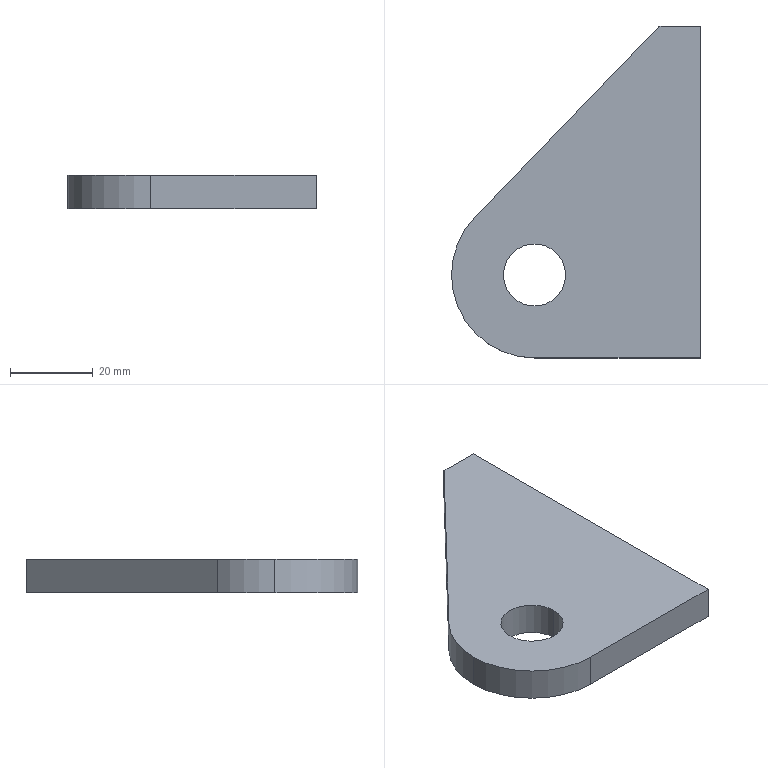Part | SolidWorks | features Extrusion 1 | 1 solid | 10 faces | box 60 x 80 x 8 mm | volume 25848 mm3 | plane 6 | cylinder 4 | commonest cylinder face diameters 15 x2 40 x2
STEP:
#1=CARTESIAN_POINT('',(-47.5,20.,4.));
#2=VERTEX_POINT('',#1);
#3=CARTESIAN_POINT('',(-32.5,20.,4.));
#4=VERTEX_POINT('',#3);
#5=CARTESIAN_POINT('',(-40.,20.,4.));
#6=DIRECTION('',(0.,0.,1.));
#7=DIRECTION('',(1.,0.,0.));
#8=AXIS2_PLACEMENT_3D('',#5,#6,#7);
#9=CIRCLE('',#8,7.5);
#10=EDGE_CURVE('',#2,#4,#9,.T.);
#11=ORIENTED_EDGE('',*,*,#10,.T.);
#12=CARTESIAN_POINT('',(-32.5,20.,-4.));
#13=VERTEX_POINT('',#12);
#14=CARTESIAN_POINT('',(-32.5,20.,4.));
#15=DIRECTION('',(0.,0.,-1.));
#16=VECTOR('',#15,1000.);
#17=LINE('',#14,#16);
#18=EDGE_CURVE('',#4,#13,#17,.T.);
#19=ORIENTED_EDGE('',*,*,#18,.T.);
#20=CARTESIAN_POINT('',(-47.5,20.,-4.));
#21=VERTEX_POINT('',#20);
#22=CARTESIAN_POINT('',(-40.,20.,-4.));
#23=DIRECTION('',(0.,0.,1.));
#24=DIRECTION('',(1.,0.,0.));
#25=AXIS2_PLACEMENT_3D('',#22,#23,#24);
#26=CIRCLE('',#25,7.5);
#27=EDGE_CURVE('',#21,#13,#26,.T.);
#28=ORIENTED_EDGE('',*,*,#27,.F.);
#29=CARTESIAN_POINT('',(-47.5,20.,4.));
#30=DIRECTION('',(0.,0.,-1.));
#31=VECTOR('',#30,1000.);
#32=LINE('',#29,#31);
#33=EDGE_CURVE('',#2,#21,#32,.T.);
#34=ORIENTED_EDGE('',*,*,#33,.F.);
#35=EDGE_LOOP('',(#11,#19,#28,#34));
#36=FACE_OUTER_BOUND('',#35,.T.);
#37=CARTESIAN_POINT('',(-40.,20.,4.));
#38=DIRECTION('',(0.,0.,-1.));
#39=DIRECTION('',(-1.,0.,0.));
#40=AXIS2_PLACEMENT_3D('',#37,#38,#39);
#41=CYLINDRICAL_SURFACE('',#40,7.5);
#42=ADVANCED_FACE('',(#36),#41,.F.);
#43=CARTESIAN_POINT('',(-60.,20.,4.));
#44=VERTEX_POINT('',#43);
#45=CARTESIAN_POINT('',(-40.,0.,4.));
#46=VERTEX_POINT('',#45);
#47=CARTESIAN_POINT('',(-40.,20.,4.));
#48=DIRECTION('',(0.,0.,1.));
#49=DIRECTION('',(1.,0.,0.));
#50=AXIS2_PLACEMENT_3D('',#47,#48,#49);
#51=CIRCLE('',#50,20.);
#52=EDGE_CURVE('',#44,#46,#51,.T.);
#53=ORIENTED_EDGE('',*,*,#52,.F.);
#54=CARTESIAN_POINT('',(-60.,20.,-4.));
#55=VERTEX_POINT('',#54);
#56=CARTESIAN_POINT('',(-60.,20.,4.));
#57=DIRECTION('',(0.,0.,-1.));
#58=VECTOR('',#57,1000.);
#59=LINE('',#56,#58);
#60=EDGE_CURVE('',#44,#55,#59,.T.);
#61=ORIENTED_EDGE('',*,*,#60,.T.);
#62=CARTESIAN_POINT('',(-40.,0.,-4.));
#63=VERTEX_POINT('',#62);
#64=CARTESIAN_POINT('',(-40.,20.,-4.));
#65=DIRECTION('',(0.,0.,1.));
#66=DIRECTION('',(1.,0.,0.));
#67=AXIS2_PLACEMENT_3D('',#64,#65,#66);
#68=CIRCLE('',#67,20.);
#69=EDGE_CURVE('',#55,#63,#68,.T.);
#70=ORIENTED_EDGE('',*,*,#69,.T.);
#71=CARTESIAN_POINT('',(-40.,0.,4.));
#72=DIRECTION('',(0.,0.,-1.));
#73=VECTOR('',#72,1000.);
#74=LINE('',#71,#73);
#75=EDGE_CURVE('',#46,#63,#74,.T.);
#76=ORIENTED_EDGE('',*,*,#75,.F.);
#77=EDGE_LOOP('',(#53,#61,#70,#76));
#78=FACE_OUTER_BOUND('',#77,.T.);
#79=CARTESIAN_POINT('',(-40.,20.,4.));
#80=DIRECTION('',(0.,0.,-1.));
#81=DIRECTION('',(-1.,0.,0.));
#82=AXIS2_PLACEMENT_3D('',#79,#80,#81);
#83=CYLINDRICAL_SURFACE('',#82,20.);
#84=ADVANCED_FACE('',(#78),#83,.T.);
#85=CARTESIAN_POINT('',(0.,0.,4.));
#86=VERTEX_POINT('',#85);
#87=CARTESIAN_POINT('',(-40.,0.,4.));
#88=DIRECTION('',(1.,0.,0.));
#89=VECTOR('',#88,1000.);
#90=LINE('',#87,#89);
#91=EDGE_CURVE('',#46,#86,#90,.T.);
#92=ORIENTED_EDGE('',*,*,#91,.T.);
#93=CARTESIAN_POINT('',(0.,80.,4.));
#94=VERTEX_POINT('',#93);
#95=CARTESIAN_POINT('',(0.,0.,4.));
#96=DIRECTION('',(0.,1.,0.));
#97=VECTOR('',#96,1000.);
#98=LINE('',#95,#97);
#99=EDGE_CURVE('',#86,#94,#98,.T.);
#100=ORIENTED_EDGE('',*,*,#99,.T.);
#101=CARTESIAN_POINT('',(-10.,80.,4.));
#102=VERTEX_POINT('',#101);
#103=CARTESIAN_POINT('',(0.,80.,4.));
#104=DIRECTION('',(-1.,0.,0.));
#105=VECTOR('',#104,1000.);
#106=LINE('',#103,#105);
#107=EDGE_CURVE('',#94,#102,#106,.T.);
#108=ORIENTED_EDGE('',*,*,#107,.T.);
#109=CARTESIAN_POINT('',(-54.408,33.871,4.));
#110=VERTEX_POINT('',#109);
#111=CARTESIAN_POINT('',(-10.,80.,4.));
#112=DIRECTION('',(-0.6935,-0.7204,0.));
#113=VECTOR('',#112,1000.);
#114=LINE('',#111,#113);
#115=EDGE_CURVE('',#102,#110,#114,.T.);
#116=ORIENTED_EDGE('',*,*,#115,.T.);
#117=CARTESIAN_POINT('',(-40.,20.,4.));
#118=DIRECTION('',(0.,0.,1.));
#119=DIRECTION('',(1.,0.,0.));
#120=AXIS2_PLACEMENT_3D('',#117,#118,#119);
#121=CIRCLE('',#120,20.);
#122=EDGE_CURVE('',#110,#44,#121,.T.);
#123=ORIENTED_EDGE('',*,*,#122,.T.);
#124=ORIENTED_EDGE('',*,*,#52,.T.);
#125=EDGE_LOOP('',(#92,#100,#108,#116,#123,#124));
#126=FACE_OUTER_BOUND('',#125,.T.);
#127=ORIENTED_EDGE('',*,*,#10,.F.);
#128=CARTESIAN_POINT('',(-40.,20.,4.));
#129=DIRECTION('',(0.,0.,1.));
#130=DIRECTION('',(1.,0.,0.));
#131=AXIS2_PLACEMENT_3D('',#128,#129,#130);
#132=CIRCLE('',#131,7.5);
#133=EDGE_CURVE('',#4,#2,#132,.T.);
#134=ORIENTED_EDGE('',*,*,#133,.F.);
#135=EDGE_LOOP('',(#127,#134));
#136=FACE_BOUND('',#135,.T.);
#137=CARTESIAN_POINT('',(-40.,20.,4.));
#138=DIRECTION('',(0.,0.,1.));
#139=DIRECTION('',(1.,0.,0.));
#140=AXIS2_PLACEMENT_3D('',#137,#138,#139);
#141=PLANE('',#140);
#142=ADVANCED_FACE('',(#126,#136),#141,.T.);
#143=CARTESIAN_POINT('',(0.,0.,-4.));
#144=VERTEX_POINT('',#143);
#145=CARTESIAN_POINT('',(-40.,0.,-4.));
#146=DIRECTION('',(1.,0.,0.));
#147=VECTOR('',#146,1000.);
#148=LINE('',#145,#147);
#149=EDGE_CURVE('',#63,#144,#148,.T.);
#150=ORIENTED_EDGE('',*,*,#149,.F.);
#151=ORIENTED_EDGE('',*,*,#69,.F.);
#152=CARTESIAN_POINT('',(-54.408,33.871,-4.));
#153=VERTEX_POINT('',#152);
#154=CARTESIAN_POINT('',(-40.,20.,-4.));
#155=DIRECTION('',(0.,0.,1.));
#156=DIRECTION('',(1.,0.,0.));
#157=AXIS2_PLACEMENT_3D('',#154,#155,#156);
#158=CIRCLE('',#157,20.);
#159=EDGE_CURVE('',#153,#55,#158,.T.);
#160=ORIENTED_EDGE('',*,*,#159,.F.);
#161=CARTESIAN_POINT('',(-10.,80.,-4.));
#162=VERTEX_POINT('',#161);
#163=CARTESIAN_POINT('',(-10.,80.,-4.));
#164=DIRECTION('',(-0.6935,-0.7204,0.));
#165=VECTOR('',#164,1000.);
#166=LINE('',#163,#165);
#167=EDGE_CURVE('',#162,#153,#166,.T.);
#168=ORIENTED_EDGE('',*,*,#167,.F.);
#169=CARTESIAN_POINT('',(0.,80.,-4.));
#170=VERTEX_POINT('',#169);
#171=CARTESIAN_POINT('',(0.,80.,-4.));
#172=DIRECTION('',(-1.,0.,0.));
#173=VECTOR('',#172,1000.);
#174=LINE('',#171,#173);
#175=EDGE_CURVE('',#170,#162,#174,.T.);
#176=ORIENTED_EDGE('',*,*,#175,.F.);
#177=CARTESIAN_POINT('',(0.,0.,-4.));
#178=DIRECTION('',(0.,1.,0.));
#179=VECTOR('',#178,1000.);
#180=LINE('',#177,#179);
#181=EDGE_CURVE('',#144,#170,#180,.T.);
#182=ORIENTED_EDGE('',*,*,#181,.F.);
#183=EDGE_LOOP('',(#150,#151,#160,#168,#176,#182));
#184=FACE_OUTER_BOUND('',#183,.T.);
#185=ORIENTED_EDGE('',*,*,#27,.T.);
#186=CARTESIAN_POINT('',(-40.,20.,-4.));
#187=DIRECTION('',(0.,0.,1.));
#188=DIRECTION('',(1.,0.,0.));
#189=AXIS2_PLACEMENT_3D('',#186,#187,#188);
#190=CIRCLE('',#189,7.5);
#191=EDGE_CURVE('',#13,#21,#190,.T.);
#192=ORIENTED_EDGE('',*,*,#191,.T.);
#193=EDGE_LOOP('',(#185,#192));
#194=FACE_BOUND('',#193,.T.);
#195=CARTESIAN_POINT('',(-40.,20.,-4.));
#196=DIRECTION('',(0.,0.,1.));
#197=DIRECTION('',(1.,0.,0.));
#198=AXIS2_PLACEMENT_3D('',#195,#196,#197);
#199=PLANE('',#198);
#200=ADVANCED_FACE('',(#184,#194),#199,.F.);
#201=ORIENTED_EDGE('',*,*,#149,.T.);
#202=CARTESIAN_POINT('',(0.,0.,4.));
#203=DIRECTION('',(0.,0.,-1.));
#204=VECTOR('',#203,1000.);
#205=LINE('',#202,#204);
#206=EDGE_CURVE('',#86,#144,#205,.T.);
#207=ORIENTED_EDGE('',*,*,#206,.F.);
#208=ORIENTED_EDGE('',*,*,#91,.F.);
#209=ORIENTED_EDGE('',*,*,#75,.T.);
#210=EDGE_LOOP('',(#201,#207,#208,#209));
#211=FACE_OUTER_BOUND('',#210,.T.);
#212=CARTESIAN_POINT('',(-40.,0.,4.));
#213=DIRECTION('',(0.,1.,0.));
#214=DIRECTION('',(0.,0.,1.));
#215=AXIS2_PLACEMENT_3D('',#212,#213,#214);
#216=PLANE('',#215);
#217=ADVANCED_FACE('',(#211),#216,.F.);
#218=ORIENTED_EDGE('',*,*,#181,.T.);
#219=CARTESIAN_POINT('',(0.,80.,4.));
#220=DIRECTION('',(0.,0.,-1.));
#221=VECTOR('',#220,1000.);
#222=LINE('',#219,#221);
#223=EDGE_CURVE('',#94,#170,#222,.T.);
#224=ORIENTED_EDGE('',*,*,#223,.F.);
#225=ORIENTED_EDGE('',*,*,#99,.F.);
#226=ORIENTED_EDGE('',*,*,#206,.T.);
#227=EDGE_LOOP('',(#218,#224,#225,#226));
#228=FACE_OUTER_BOUND('',#227,.T.);
#229=CARTESIAN_POINT('',(0.,0.,4.));
#230=DIRECTION('',(-1.,0.,0.));
#231=DIRECTION('',(0.,0.,1.));
#232=AXIS2_PLACEMENT_3D('',#229,#230,#231);
#233=PLANE('',#232);
#234=ADVANCED_FACE('',(#228),#233,.F.);
#235=ORIENTED_EDGE('',*,*,#175,.T.);
#236=CARTESIAN_POINT('',(-10.,80.,4.));
#237=DIRECTION('',(0.,0.,-1.));
#238=VECTOR('',#237,1000.);
#239=LINE('',#236,#238);
#240=EDGE_CURVE('',#102,#162,#239,.T.);
#241=ORIENTED_EDGE('',*,*,#240,.F.);
#242=ORIENTED_EDGE('',*,*,#107,.F.);
#243=ORIENTED_EDGE('',*,*,#223,.T.);
#244=EDGE_LOOP('',(#235,#241,#242,#243));
#245=FACE_OUTER_BOUND('',#244,.T.);
#246=CARTESIAN_POINT('',(0.,80.,4.));
#247=DIRECTION('',(0.,-1.,0.));
#248=DIRECTION('',(0.,0.,-1.));
#249=AXIS2_PLACEMENT_3D('',#246,#247,#248);
#250=PLANE('',#249);
#251=ADVANCED_FACE('',(#245),#250,.F.);
#252=ORIENTED_EDGE('',*,*,#167,.T.);
#253=CARTESIAN_POINT('',(-54.408,33.871,4.));
#254=DIRECTION('',(0.,0.,-1.));
#255=VECTOR('',#254,1000.);
#256=LINE('',#253,#255);
#257=EDGE_CURVE('',#110,#153,#256,.T.);
#258=ORIENTED_EDGE('',*,*,#257,.F.);
#259=ORIENTED_EDGE('',*,*,#115,.F.);
#260=ORIENTED_EDGE('',*,*,#240,.T.);
#261=EDGE_LOOP('',(#252,#258,#259,#260));
#262=FACE_OUTER_BOUND('',#261,.T.);
#263=CARTESIAN_POINT('',(-10.,80.,4.));
#264=DIRECTION('',(0.7204,-0.6935,0.));
#265=DIRECTION('',(0.6935,0.7204,0.));
#266=AXIS2_PLACEMENT_3D('',#263,#264,#265);
#267=PLANE('',#266);
#268=ADVANCED_FACE('',(#262),#267,.F.);
#269=ORIENTED_EDGE('',*,*,#60,.F.);
#270=ORIENTED_EDGE('',*,*,#122,.F.);
#271=ORIENTED_EDGE('',*,*,#257,.T.);
#272=ORIENTED_EDGE('',*,*,#159,.T.);
#273=EDGE_LOOP('',(#269,#270,#271,#272));
#274=FACE_OUTER_BOUND('',#273,.T.);
#275=CARTESIAN_POINT('',(-40.,20.,4.));
#276=DIRECTION('',(0.,0.,-1.));
#277=DIRECTION('',(-1.,0.,0.));
#278=AXIS2_PLACEMENT_3D('',#275,#276,#277);
#279=CYLINDRICAL_SURFACE('',#278,20.);
#280=ADVANCED_FACE('',(#274),#279,.T.);
#281=ORIENTED_EDGE('',*,*,#18,.F.);
#282=ORIENTED_EDGE('',*,*,#133,.T.);
#283=ORIENTED_EDGE('',*,*,#33,.T.);
#284=ORIENTED_EDGE('',*,*,#191,.F.);
#285=EDGE_LOOP('',(#281,#282,#283,#284));
#286=FACE_OUTER_BOUND('',#285,.T.);
#287=CARTESIAN_POINT('',(-40.,20.,4.));
#288=DIRECTION('',(0.,0.,-1.));
#289=DIRECTION('',(-1.,0.,0.));
#290=AXIS2_PLACEMENT_3D('',#287,#288,#289);
#291=CYLINDRICAL_SURFACE('',#290,7.5);
#292=ADVANCED_FACE('',(#286),#291,.F.);
#293=CLOSED_SHELL('',(#42,#84,#142,#200,#217,#234,#251,#268,#280,#292));
#294=MANIFOLD_SOLID_BREP('',#293);
#295=CARTESIAN_POINT('',(0.,0.,0.));
#296=DIRECTION('',(0.,0.,1.));
#297=DIRECTION('',(1.,0.,0.));
#298=AXIS2_PLACEMENT_3D('',#295,#296,#297);
#299=(LENGTH_UNIT()NAMED_UNIT(*)SI_UNIT(.MILLI.,.METRE.));
#300=UNCERTAINTY_MEASURE_WITH_UNIT(LENGTH_MEASURE(0.00001),#299,'','');
#301=(NAMED_UNIT(*)PLANE_ANGLE_UNIT()SI_UNIT($,.RADIAN.));
#302=(NAMED_UNIT(*)SI_UNIT($,.STERADIAN.)SOLID_ANGLE_UNIT());
#303=(GEOMETRIC_REPRESENTATION_CONTEXT(3)GLOBAL_UNCERTAINTY_ASSIGNED_CONTEXT((#300))GLOBAL_UNIT_ASSIGNED_CONTEXT((#299,#301,#302))REPRESENTATION_CONTEXT('',''));
#304=ADVANCED_BREP_SHAPE_REPRESENTATION('',(#294,#298),#303);